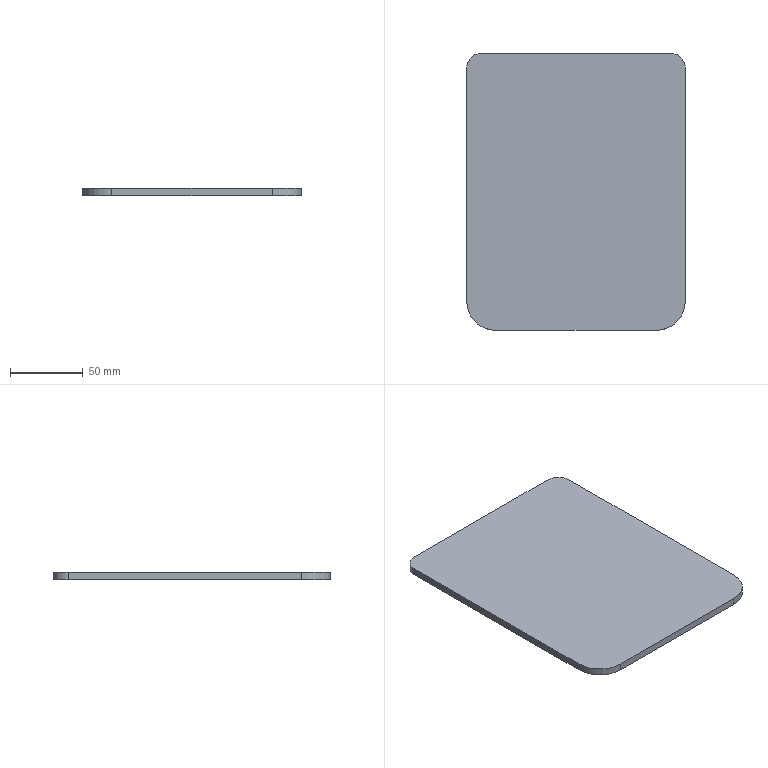Part | SolidWorks | features Fillet 2, Extrusion 1 | 1 solid | 10 faces | box 150 x 190 x 5 mm | volume 141427 mm3 | plane 6 | cylinder 4 | commonest cylinder face diameters 20 x2 40 x2
STEP:
#1=CARTESIAN_POINT('',(75.,-75.,5.));
#2=VERTEX_POINT('',#1);
#3=CARTESIAN_POINT('',(75.,85.,5.));
#4=VERTEX_POINT('',#3);
#5=CARTESIAN_POINT('',(75.,95.,5.));
#6=DIRECTION('',(0.,1.,0.));
#7=VECTOR('',#6,1000.);
#8=LINE('',#5,#7);
#9=EDGE_CURVE('',#2,#4,#8,.T.);
#10=ORIENTED_EDGE('',*,*,#9,.F.);
#11=CARTESIAN_POINT('',(75.,-75.,0.));
#12=VERTEX_POINT('',#11);
#13=CARTESIAN_POINT('',(75.,-75.,5.));
#14=DIRECTION('',(0.,0.,-1.));
#15=VECTOR('',#14,1000.);
#16=LINE('',#13,#15);
#17=EDGE_CURVE('',#2,#12,#16,.T.);
#18=ORIENTED_EDGE('',*,*,#17,.T.);
#19=CARTESIAN_POINT('',(75.,85.,0.));
#20=VERTEX_POINT('',#19);
#21=CARTESIAN_POINT('',(75.,95.,0.));
#22=DIRECTION('',(0.,1.,0.));
#23=VECTOR('',#22,1000.);
#24=LINE('',#21,#23);
#25=EDGE_CURVE('',#12,#20,#24,.T.);
#26=ORIENTED_EDGE('',*,*,#25,.T.);
#27=CARTESIAN_POINT('',(75.,85.,5.));
#28=DIRECTION('',(0.,0.,1.));
#29=VECTOR('',#28,1000.);
#30=LINE('',#27,#29);
#31=EDGE_CURVE('',#20,#4,#30,.T.);
#32=ORIENTED_EDGE('',*,*,#31,.T.);
#33=EDGE_LOOP('',(#10,#18,#26,#32));
#34=FACE_OUTER_BOUND('',#33,.T.);
#35=CARTESIAN_POINT('',(75.,95.,5.));
#36=DIRECTION('',(-1.,0.,0.));
#37=DIRECTION('',(0.,-1.,0.));
#38=AXIS2_PLACEMENT_3D('',#35,#36,#37);
#39=PLANE('',#38);
#40=ADVANCED_FACE('',(#34),#39,.F.);
#41=CARTESIAN_POINT('',(65.,95.,0.));
#42=VERTEX_POINT('',#41);
#43=CARTESIAN_POINT('',(-65.,95.,0.));
#44=VERTEX_POINT('',#43);
#45=CARTESIAN_POINT('',(-75.,95.,0.));
#46=DIRECTION('',(-1.,0.,0.));
#47=VECTOR('',#46,1000.);
#48=LINE('',#45,#47);
#49=EDGE_CURVE('',#42,#44,#48,.T.);
#50=ORIENTED_EDGE('',*,*,#49,.T.);
#51=CARTESIAN_POINT('',(-65.,95.,5.));
#52=VERTEX_POINT('',#51);
#53=CARTESIAN_POINT('',(-65.,95.,5.));
#54=DIRECTION('',(0.,0.,1.));
#55=VECTOR('',#54,1000.);
#56=LINE('',#53,#55);
#57=EDGE_CURVE('',#44,#52,#56,.T.);
#58=ORIENTED_EDGE('',*,*,#57,.T.);
#59=CARTESIAN_POINT('',(65.,95.,5.));
#60=VERTEX_POINT('',#59);
#61=CARTESIAN_POINT('',(-75.,95.,5.));
#62=DIRECTION('',(-1.,0.,0.));
#63=VECTOR('',#62,1000.);
#64=LINE('',#61,#63);
#65=EDGE_CURVE('',#60,#52,#64,.T.);
#66=ORIENTED_EDGE('',*,*,#65,.F.);
#67=CARTESIAN_POINT('',(65.,95.,5.));
#68=DIRECTION('',(0.,0.,-1.));
#69=VECTOR('',#68,1000.);
#70=LINE('',#67,#69);
#71=EDGE_CURVE('',#60,#42,#70,.T.);
#72=ORIENTED_EDGE('',*,*,#71,.T.);
#73=EDGE_LOOP('',(#50,#58,#66,#72));
#74=FACE_OUTER_BOUND('',#73,.T.);
#75=CARTESIAN_POINT('',(-75.,95.,5.));
#76=DIRECTION('',(0.,-1.,0.));
#77=DIRECTION('',(0.,0.,-1.));
#78=AXIS2_PLACEMENT_3D('',#75,#76,#77);
#79=PLANE('',#78);
#80=ADVANCED_FACE('',(#74),#79,.F.);
#81=CARTESIAN_POINT('',(-75.,85.,0.));
#82=VERTEX_POINT('',#81);
#83=CARTESIAN_POINT('',(-75.,-75.,0.));
#84=VERTEX_POINT('',#83);
#85=CARTESIAN_POINT('',(-75.,95.,0.));
#86=DIRECTION('',(0.,-1.,0.));
#87=VECTOR('',#86,1000.);
#88=LINE('',#85,#87);
#89=EDGE_CURVE('',#82,#84,#88,.T.);
#90=ORIENTED_EDGE('',*,*,#89,.T.);
#91=CARTESIAN_POINT('',(-75.,-75.,5.));
#92=VERTEX_POINT('',#91);
#93=CARTESIAN_POINT('',(-75.,-75.,5.));
#94=DIRECTION('',(0.,0.,1.));
#95=VECTOR('',#94,1000.);
#96=LINE('',#93,#95);
#97=EDGE_CURVE('',#84,#92,#96,.T.);
#98=ORIENTED_EDGE('',*,*,#97,.T.);
#99=CARTESIAN_POINT('',(-75.,85.,5.));
#100=VERTEX_POINT('',#99);
#101=CARTESIAN_POINT('',(-75.,95.,5.));
#102=DIRECTION('',(0.,-1.,0.));
#103=VECTOR('',#102,1000.);
#104=LINE('',#101,#103);
#105=EDGE_CURVE('',#100,#92,#104,.T.);
#106=ORIENTED_EDGE('',*,*,#105,.F.);
#107=CARTESIAN_POINT('',(-75.,85.,5.));
#108=DIRECTION('',(0.,0.,-1.));
#109=VECTOR('',#108,1000.);
#110=LINE('',#107,#109);
#111=EDGE_CURVE('',#100,#82,#110,.T.);
#112=ORIENTED_EDGE('',*,*,#111,.T.);
#113=EDGE_LOOP('',(#90,#98,#106,#112));
#114=FACE_OUTER_BOUND('',#113,.T.);
#115=CARTESIAN_POINT('',(-75.,95.,5.));
#116=DIRECTION('',(1.,0.,0.));
#117=DIRECTION('',(0.,1.,0.));
#118=AXIS2_PLACEMENT_3D('',#115,#116,#117);
#119=PLANE('',#118);
#120=ADVANCED_FACE('',(#114),#119,.F.);
#121=CARTESIAN_POINT('',(-55.,-95.,5.));
#122=VERTEX_POINT('',#121);
#123=CARTESIAN_POINT('',(55.,-95.,5.));
#124=VERTEX_POINT('',#123);
#125=CARTESIAN_POINT('',(-75.,-95.,5.));
#126=DIRECTION('',(1.,0.,0.));
#127=VECTOR('',#126,1000.);
#128=LINE('',#125,#127);
#129=EDGE_CURVE('',#122,#124,#128,.T.);
#130=ORIENTED_EDGE('',*,*,#129,.F.);
#131=CARTESIAN_POINT('',(-55.,-95.,0.));
#132=VERTEX_POINT('',#131);
#133=CARTESIAN_POINT('',(-55.,-95.,5.));
#134=DIRECTION('',(0.,0.,-1.));
#135=VECTOR('',#134,1000.);
#136=LINE('',#133,#135);
#137=EDGE_CURVE('',#122,#132,#136,.T.);
#138=ORIENTED_EDGE('',*,*,#137,.T.);
#139=CARTESIAN_POINT('',(55.,-95.,0.));
#140=VERTEX_POINT('',#139);
#141=CARTESIAN_POINT('',(-75.,-95.,0.));
#142=DIRECTION('',(1.,0.,0.));
#143=VECTOR('',#142,1000.);
#144=LINE('',#141,#143);
#145=EDGE_CURVE('',#132,#140,#144,.T.);
#146=ORIENTED_EDGE('',*,*,#145,.T.);
#147=CARTESIAN_POINT('',(55.,-95.,5.));
#148=DIRECTION('',(0.,0.,1.));
#149=VECTOR('',#148,1000.);
#150=LINE('',#147,#149);
#151=EDGE_CURVE('',#140,#124,#150,.T.);
#152=ORIENTED_EDGE('',*,*,#151,.T.);
#153=EDGE_LOOP('',(#130,#138,#146,#152));
#154=FACE_OUTER_BOUND('',#153,.T.);
#155=CARTESIAN_POINT('',(-75.,-95.,5.));
#156=DIRECTION('',(0.,1.,0.));
#157=DIRECTION('',(0.,0.,1.));
#158=AXIS2_PLACEMENT_3D('',#155,#156,#157);
#159=PLANE('',#158);
#160=ADVANCED_FACE('',(#154),#159,.F.);
#161=ORIENTED_EDGE('',*,*,#105,.T.);
#162=CARTESIAN_POINT('',(-55.,-75.,5.));
#163=DIRECTION('',(0.,0.,1.));
#164=DIRECTION('',(1.,0.,0.));
#165=AXIS2_PLACEMENT_3D('',#162,#163,#164);
#166=CIRCLE('',#165,20.);
#167=EDGE_CURVE('',#92,#122,#166,.T.);
#168=ORIENTED_EDGE('',*,*,#167,.T.);
#169=ORIENTED_EDGE('',*,*,#129,.T.);
#170=CARTESIAN_POINT('',(55.,-75.,5.));
#171=DIRECTION('',(0.,0.,1.));
#172=DIRECTION('',(1.,0.,0.));
#173=AXIS2_PLACEMENT_3D('',#170,#171,#172);
#174=CIRCLE('',#173,20.);
#175=EDGE_CURVE('',#124,#2,#174,.T.);
#176=ORIENTED_EDGE('',*,*,#175,.T.);
#177=ORIENTED_EDGE('',*,*,#9,.T.);
#178=CARTESIAN_POINT('',(65.,85.,5.));
#179=DIRECTION('',(0.,0.,1.));
#180=DIRECTION('',(1.,0.,0.));
#181=AXIS2_PLACEMENT_3D('',#178,#179,#180);
#182=CIRCLE('',#181,10.);
#183=EDGE_CURVE('',#4,#60,#182,.T.);
#184=ORIENTED_EDGE('',*,*,#183,.T.);
#185=ORIENTED_EDGE('',*,*,#65,.T.);
#186=CARTESIAN_POINT('',(-65.,85.,5.));
#187=DIRECTION('',(0.,0.,1.));
#188=DIRECTION('',(1.,0.,0.));
#189=AXIS2_PLACEMENT_3D('',#186,#187,#188);
#190=CIRCLE('',#189,10.);
#191=EDGE_CURVE('',#52,#100,#190,.T.);
#192=ORIENTED_EDGE('',*,*,#191,.T.);
#193=EDGE_LOOP('',(#161,#168,#169,#176,#177,#184,#185,#192));
#194=FACE_OUTER_BOUND('',#193,.T.);
#195=CARTESIAN_POINT('',(0.,0.,5.));
#196=DIRECTION('',(0.,0.,1.));
#197=DIRECTION('',(1.,0.,0.));
#198=AXIS2_PLACEMENT_3D('',#195,#196,#197);
#199=PLANE('',#198);
#200=ADVANCED_FACE('',(#194),#199,.T.);
#201=ORIENTED_EDGE('',*,*,#145,.F.);
#202=CARTESIAN_POINT('',(-55.,-75.,0.));
#203=DIRECTION('',(0.,0.,-1.));
#204=DIRECTION('',(1.,0.,0.));
#205=AXIS2_PLACEMENT_3D('',#202,#203,#204);
#206=CIRCLE('',#205,20.);
#207=EDGE_CURVE('',#132,#84,#206,.T.);
#208=ORIENTED_EDGE('',*,*,#207,.T.);
#209=ORIENTED_EDGE('',*,*,#89,.F.);
#210=CARTESIAN_POINT('',(-65.,85.,0.));
#211=DIRECTION('',(0.,0.,-1.));
#212=DIRECTION('',(1.,0.,0.));
#213=AXIS2_PLACEMENT_3D('',#210,#211,#212);
#214=CIRCLE('',#213,10.);
#215=EDGE_CURVE('',#82,#44,#214,.T.);
#216=ORIENTED_EDGE('',*,*,#215,.T.);
#217=ORIENTED_EDGE('',*,*,#49,.F.);
#218=CARTESIAN_POINT('',(65.,85.,0.));
#219=DIRECTION('',(0.,0.,-1.));
#220=DIRECTION('',(1.,0.,0.));
#221=AXIS2_PLACEMENT_3D('',#218,#219,#220);
#222=CIRCLE('',#221,10.);
#223=EDGE_CURVE('',#42,#20,#222,.T.);
#224=ORIENTED_EDGE('',*,*,#223,.T.);
#225=ORIENTED_EDGE('',*,*,#25,.F.);
#226=CARTESIAN_POINT('',(55.,-75.,0.));
#227=DIRECTION('',(0.,0.,-1.));
#228=DIRECTION('',(1.,0.,0.));
#229=AXIS2_PLACEMENT_3D('',#226,#227,#228);
#230=CIRCLE('',#229,20.);
#231=EDGE_CURVE('',#12,#140,#230,.T.);
#232=ORIENTED_EDGE('',*,*,#231,.T.);
#233=EDGE_LOOP('',(#201,#208,#209,#216,#217,#224,#225,#232));
#234=FACE_OUTER_BOUND('',#233,.T.);
#235=CARTESIAN_POINT('',(0.,0.,0.));
#236=DIRECTION('',(0.,0.,1.));
#237=DIRECTION('',(1.,0.,0.));
#238=AXIS2_PLACEMENT_3D('',#235,#236,#237);
#239=PLANE('',#238);
#240=ADVANCED_FACE('',(#234),#239,.F.);
#241=ORIENTED_EDGE('',*,*,#191,.F.);
#242=ORIENTED_EDGE('',*,*,#57,.F.);
#243=ORIENTED_EDGE('',*,*,#215,.F.);
#244=ORIENTED_EDGE('',*,*,#111,.F.);
#245=EDGE_LOOP('',(#241,#242,#243,#244));
#246=FACE_OUTER_BOUND('',#245,.T.);
#247=CARTESIAN_POINT('',(-65.,85.,5.));
#248=DIRECTION('',(0.,0.,-1.));
#249=DIRECTION('',(-1.,0.,0.));
#250=AXIS2_PLACEMENT_3D('',#247,#248,#249);
#251=CYLINDRICAL_SURFACE('',#250,10.);
#252=ADVANCED_FACE('',(#246),#251,.T.);
#253=ORIENTED_EDGE('',*,*,#183,.F.);
#254=ORIENTED_EDGE('',*,*,#31,.F.);
#255=ORIENTED_EDGE('',*,*,#223,.F.);
#256=ORIENTED_EDGE('',*,*,#71,.F.);
#257=EDGE_LOOP('',(#253,#254,#255,#256));
#258=FACE_OUTER_BOUND('',#257,.T.);
#259=CARTESIAN_POINT('',(65.,85.,5.));
#260=DIRECTION('',(0.,0.,-1.));
#261=DIRECTION('',(-1.,0.,0.));
#262=AXIS2_PLACEMENT_3D('',#259,#260,#261);
#263=CYLINDRICAL_SURFACE('',#262,10.);
#264=ADVANCED_FACE('',(#258),#263,.T.);
#265=ORIENTED_EDGE('',*,*,#167,.F.);
#266=ORIENTED_EDGE('',*,*,#97,.F.);
#267=ORIENTED_EDGE('',*,*,#207,.F.);
#268=ORIENTED_EDGE('',*,*,#137,.F.);
#269=EDGE_LOOP('',(#265,#266,#267,#268));
#270=FACE_OUTER_BOUND('',#269,.T.);
#271=CARTESIAN_POINT('',(-55.,-75.,5.));
#272=DIRECTION('',(0.,0.,-1.));
#273=DIRECTION('',(-1.,0.,0.));
#274=AXIS2_PLACEMENT_3D('',#271,#272,#273);
#275=CYLINDRICAL_SURFACE('',#274,20.);
#276=ADVANCED_FACE('',(#270),#275,.T.);
#277=ORIENTED_EDGE('',*,*,#175,.F.);
#278=ORIENTED_EDGE('',*,*,#151,.F.);
#279=ORIENTED_EDGE('',*,*,#231,.F.);
#280=ORIENTED_EDGE('',*,*,#17,.F.);
#281=EDGE_LOOP('',(#277,#278,#279,#280));
#282=FACE_OUTER_BOUND('',#281,.T.);
#283=CARTESIAN_POINT('',(55.,-75.,5.));
#284=DIRECTION('',(0.,0.,-1.));
#285=DIRECTION('',(-1.,0.,0.));
#286=AXIS2_PLACEMENT_3D('',#283,#284,#285);
#287=CYLINDRICAL_SURFACE('',#286,20.);
#288=ADVANCED_FACE('',(#282),#287,.T.);
#289=CLOSED_SHELL('',(#40,#80,#120,#160,#200,#240,#252,#264,#276,#288));
#290=MANIFOLD_SOLID_BREP('',#289);
#291=CARTESIAN_POINT('',(0.,0.,0.));
#292=DIRECTION('',(0.,0.,1.));
#293=DIRECTION('',(1.,0.,0.));
#294=AXIS2_PLACEMENT_3D('',#291,#292,#293);
#295=(LENGTH_UNIT()NAMED_UNIT(*)SI_UNIT(.MILLI.,.METRE.));
#296=UNCERTAINTY_MEASURE_WITH_UNIT(LENGTH_MEASURE(0.00001),#295,'','');
#297=(NAMED_UNIT(*)PLANE_ANGLE_UNIT()SI_UNIT($,.RADIAN.));
#298=(NAMED_UNIT(*)SI_UNIT($,.STERADIAN.)SOLID_ANGLE_UNIT());
#299=(GEOMETRIC_REPRESENTATION_CONTEXT(3)GLOBAL_UNCERTAINTY_ASSIGNED_CONTEXT((#296))GLOBAL_UNIT_ASSIGNED_CONTEXT((#295,#297,#298))REPRESENTATION_CONTEXT('',''));
#300=ADVANCED_BREP_SHAPE_REPRESENTATION('',(#290,#294),#299);